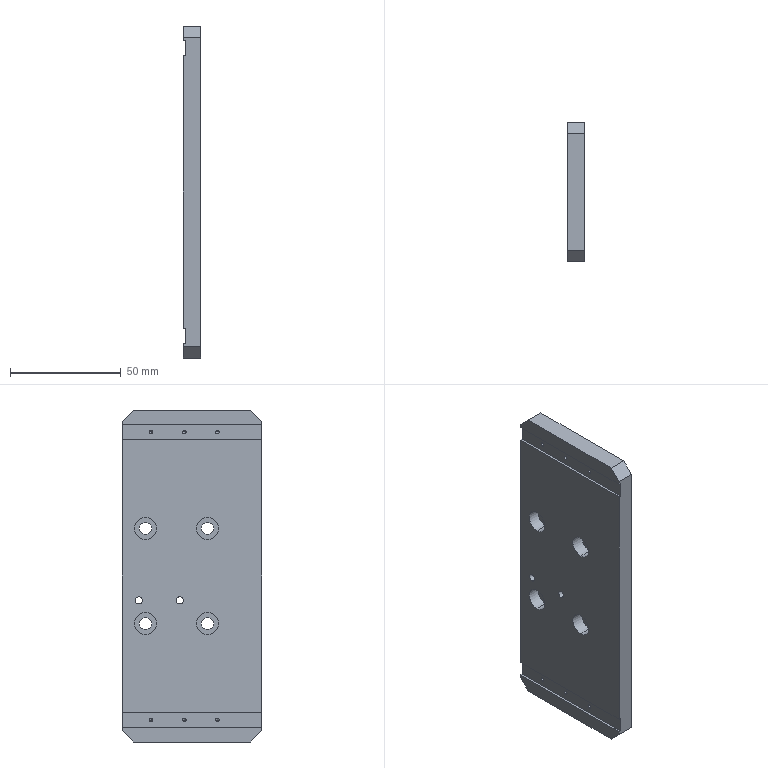Part | SolidWorks | features HoleWzd 3, Chamfer 1, Extrusion 1, ICE 1 | 1 solid | 74 faces | box 8 x 63 x 150 mm | volume 72107 mm3 | cylinder 32 | plane 22 | cone 20 | commonest cylinder face diameters 1.6 x12 5.5 x8 10 x8 3.3 x4